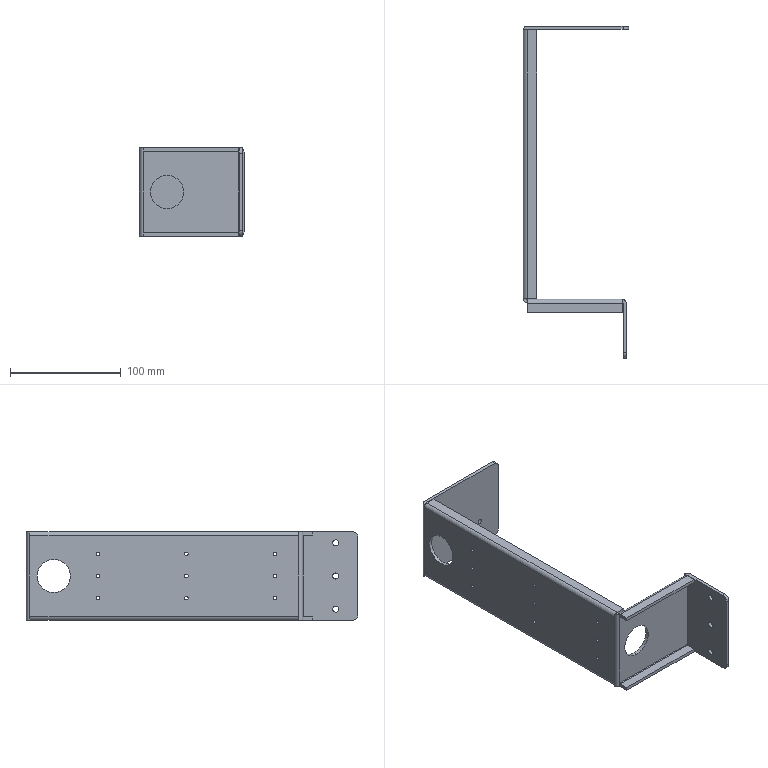Part | SolidWorks | features BaseBody 1 | 1 solid | 94 faces | box 95 x 300 x 80 mm | volume 126300 mm3 | cylinder 50 | plane 44 | commonest cylinder face diameters 3.3 x18 1 x7 7 x7 5.5 x6 4.2 x4 10 x4